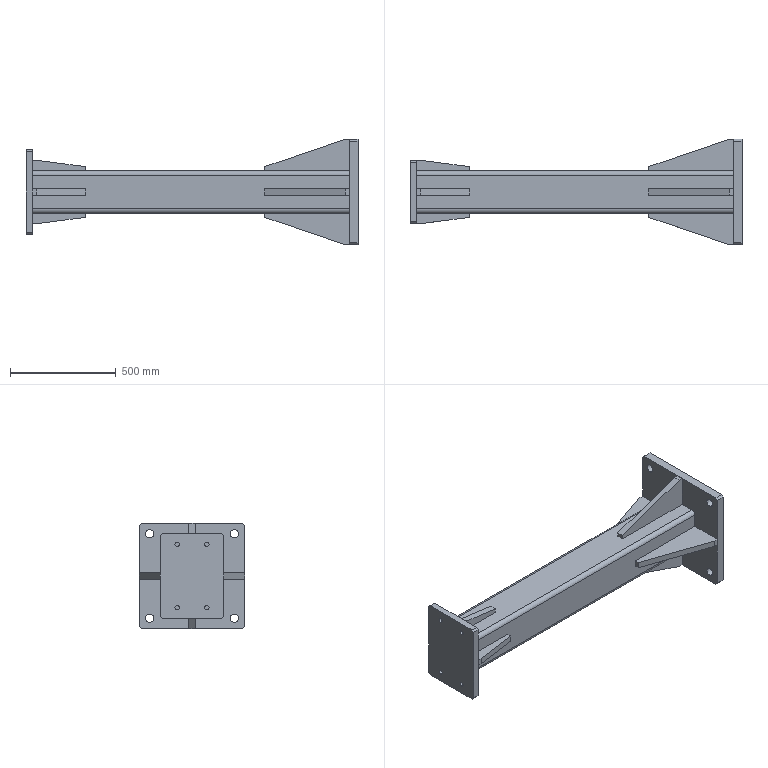Part | SolidWorks | features ICE 3, Chamfer 2, CirPattern 2, HoleWzd 2, Split 2, CombineBodies 1, Rib 1, WeldMemberFeat 1, WeldmentFeature 1 | 7 solids | 107 faces | box 1570 x 500 x 500 mm | volume 29641235 mm3 | plane 81 | cylinder 26 | commonest cylinder face diameters 39 x10 21 x8 20 x4 40 x4